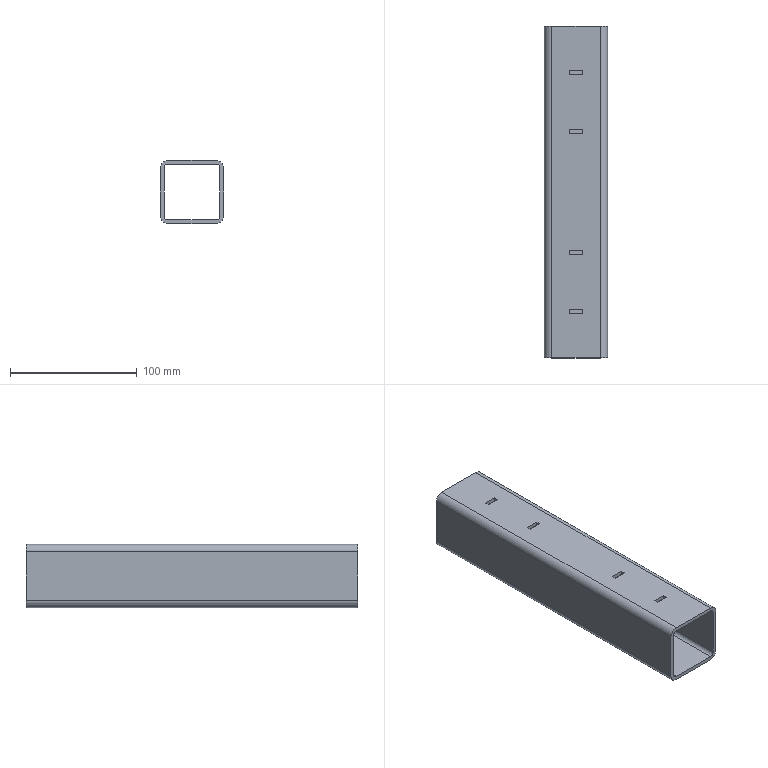Part | SolidWorks | features BaseBody 1 | 1 solid | 83 faces | box 50 x 262 x 50 mm | volume 141281 mm3 | plane 46 | spline 29 | cylinder 8 | commonest cylinder face diameters 6 x4 12 x4